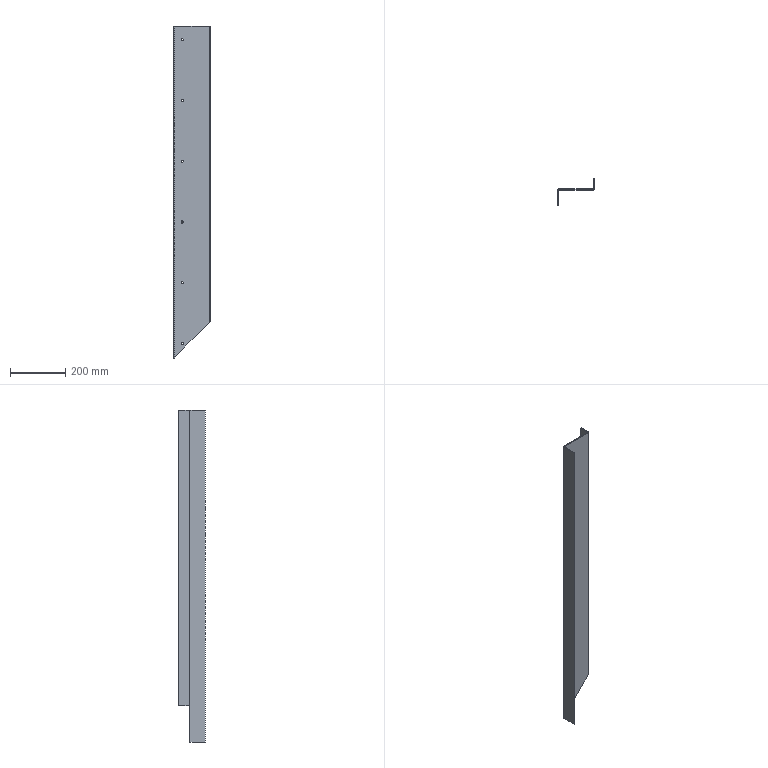Part | STEP file | TS-Z001-07 | 1 solid | 35 faces | box 131 x 95 x 1203 mm | volume 758625 mm3 | plane 17 | cylinder 16 | spline 2 | commonest cylinder face diameters 8 x12 0.4 x2 6.4 x2